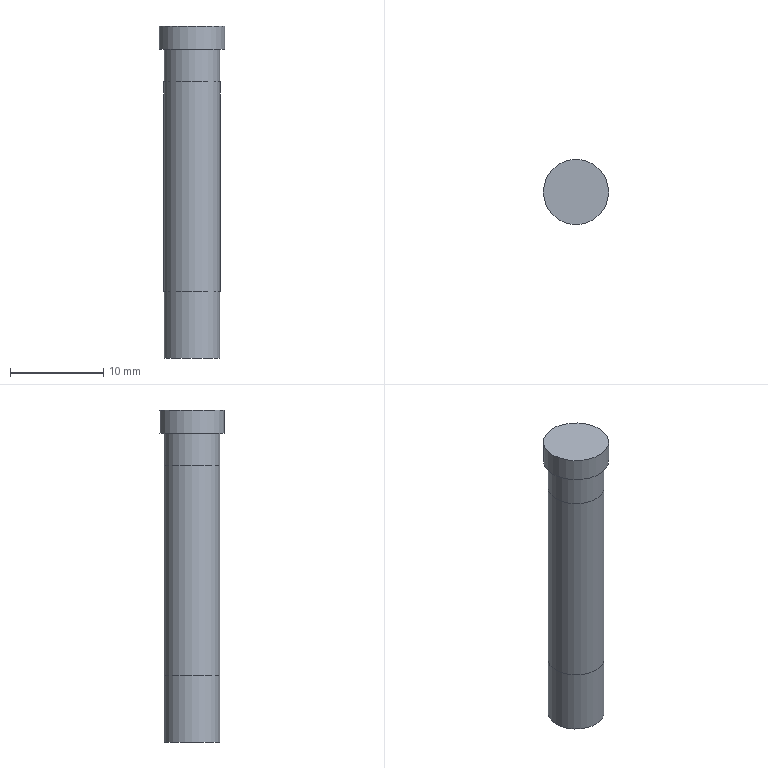Part | NX | features BREP 2 | 2 solids | 10 faces | box 7 x 7 x 35.6 mm | volume 1730 mm3 | plane 5 | cylinder 3 | torus 1 | cone 1 | commonest cylinder face diameters 6 x1 6.008 x1 7 x1
STEP:
#1=CARTESIAN_POINT('',(3.5,0.,-2.5));
#2=VERTEX_POINT('',#1);
#3=CARTESIAN_POINT('',(0.,0.,-2.5));
#4=DIRECTION('',(0.,0.,1.));
#5=DIRECTION('',(1.,0.,0.));
#6=AXIS2_PLACEMENT_3D('',#3,#4,#5);
#7=CIRCLE('',#6,3.5);
#8=EDGE_CURVE('',#2,#2,#7,.T.);
#9=ORIENTED_EDGE('',*,*,#8,.T.);
#10=EDGE_LOOP('',(#9));
#11=FACE_BOUND('',#10,.T.);
#12=CARTESIAN_POINT('',(3.5,0.,0.));
#13=VERTEX_POINT('',#12);
#14=CARTESIAN_POINT('',(0.,0.,0.));
#15=DIRECTION('',(0.,0.,1.));
#16=DIRECTION('',(1.,0.,0.));
#17=AXIS2_PLACEMENT_3D('',#14,#15,#16);
#18=CIRCLE('',#17,3.5);
#19=EDGE_CURVE('',#13,#13,#18,.T.);
#20=ORIENTED_EDGE('',*,*,#19,.F.);
#21=EDGE_LOOP('',(#20));
#22=FACE_BOUND('',#21,.T.);
#23=CARTESIAN_POINT('',(0.,0.,-2.5));
#24=DIRECTION('',(0.,0.,1.));
#25=DIRECTION('',(-1.,0.,0.));
#26=AXIS2_PLACEMENT_3D('',#23,#24,#25);
#27=CYLINDRICAL_SURFACE('',#26,3.5);
#28=ADVANCED_FACE('',(#11,#22),#27,.T.);
#29=CARTESIAN_POINT('',(-3.,0.,-2.5));
#30=VERTEX_POINT('',#29);
#31=CARTESIAN_POINT('',(0.,0.,-2.5));
#32=DIRECTION('',(0.,0.,-1.));
#33=DIRECTION('',(-1.,0.,0.));
#34=AXIS2_PLACEMENT_3D('',#31,#32,#33);
#35=CIRCLE('',#34,3.);
#36=EDGE_CURVE('',#30,#30,#35,.T.);
#37=ORIENTED_EDGE('',*,*,#36,.F.);
#38=EDGE_LOOP('',(#37));
#39=FACE_BOUND('',#38,.T.);
#40=ORIENTED_EDGE('',*,*,#8,.F.);
#41=EDGE_LOOP('',(#40));
#42=FACE_BOUND('',#41,.T.);
#43=CARTESIAN_POINT('',(0.,0.,-2.5));
#44=DIRECTION('',(0.,0.,1.));
#45=DIRECTION('',(-1.,0.,0.));
#46=AXIS2_PLACEMENT_3D('',#43,#44,#45);
#47=PLANE('',#46);
#48=ADVANCED_FACE('',(#39,#42),#47,.F.);
#49=ORIENTED_EDGE('',*,*,#19,.T.);
#50=EDGE_LOOP('',(#49));
#51=FACE_BOUND('',#50,.T.);
#52=CARTESIAN_POINT('',(0.,0.,0.));
#53=DIRECTION('',(0.,0.,1.));
#54=DIRECTION('',(-1.,0.,0.));
#55=AXIS2_PLACEMENT_3D('',#52,#53,#54);
#56=PLANE('',#55);
#57=ADVANCED_FACE('',(#51),#56,.T.);
#58=ORIENTED_EDGE('',*,*,#36,.T.);
#59=EDGE_LOOP('',(#58));
#60=FACE_BOUND('',#59,.T.);
#61=CARTESIAN_POINT('',(-3.,0.,-35.6));
#62=VERTEX_POINT('',#61);
#63=CARTESIAN_POINT('',(0.,0.,-35.6));
#64=DIRECTION('',(0.,0.,-1.));
#65=DIRECTION('',(-1.,0.,0.));
#66=AXIS2_PLACEMENT_3D('',#63,#64,#65);
#67=CIRCLE('',#66,3.);
#68=EDGE_CURVE('',#62,#62,#67,.T.);
#69=ORIENTED_EDGE('',*,*,#68,.F.);
#70=EDGE_LOOP('',(#69));
#71=FACE_BOUND('',#70,.T.);
#72=CARTESIAN_POINT('',(0.,0.,-2.5));
#73=DIRECTION('',(0.,0.,-1.));
#74=DIRECTION('',(1.,0.,0.));
#75=AXIS2_PLACEMENT_3D('',#72,#73,#74);
#76=CYLINDRICAL_SURFACE('',#75,3.);
#77=ADVANCED_FACE('',(#60,#71),#76,.T.);
#78=ORIENTED_EDGE('',*,*,#68,.T.);
#79=EDGE_LOOP('',(#78));
#80=FACE_BOUND('',#79,.T.);
#81=CARTESIAN_POINT('',(0.,0.,-35.6));
#82=DIRECTION('',(0.,0.,-1.));
#83=DIRECTION('',(1.,0.,0.));
#84=AXIS2_PLACEMENT_3D('',#81,#82,#83);
#85=PLANE('',#84);
#86=ADVANCED_FACE('',(#80),#85,.T.);
#87=CLOSED_SHELL('',(#28,#48,#57,#77,#86));
#88=MANIFOLD_SOLID_BREP('',#87);
#89=CARTESIAN_POINT('',(3.004,0.,-28.5));
#90=VERTEX_POINT('',#89);
#91=CARTESIAN_POINT('',(0.,0.,-28.5));
#92=DIRECTION('',(0.,0.,1.));
#93=DIRECTION('',(1.,0.,0.));
#94=AXIS2_PLACEMENT_3D('',#91,#92,#93);
#95=CIRCLE('',#94,3.004);
#96=EDGE_CURVE('',#90,#90,#95,.T.);
#97=ORIENTED_EDGE('',*,*,#96,.T.);
#98=EDGE_LOOP('',(#97));
#99=FACE_BOUND('',#98,.T.);
#100=CARTESIAN_POINT('',(3.004,0.,-6.));
#101=VERTEX_POINT('',#100);
#102=CARTESIAN_POINT('',(0.,0.,-6.));
#103=DIRECTION('',(0.,0.,-1.));
#104=DIRECTION('',(1.,0.,0.));
#105=AXIS2_PLACEMENT_3D('',#102,#103,#104);
#106=CIRCLE('',#105,3.004);
#107=EDGE_CURVE('',#101,#101,#106,.T.);
#108=ORIENTED_EDGE('',*,*,#107,.T.);
#109=EDGE_LOOP('',(#108));
#110=FACE_BOUND('',#109,.T.);
#111=CARTESIAN_POINT('',(0.,0.,-29.5));
#112=DIRECTION('',(0.,0.,1.));
#113=DIRECTION('',(-1.,0.,0.));
#114=AXIS2_PLACEMENT_3D('',#111,#112,#113);
#115=CYLINDRICAL_SURFACE('',#114,3.004);
#116=ADVANCED_FACE('',(#99,#110),#115,.T.);
#117=CARTESIAN_POINT('',(2.736,0.,-29.5));
#118=VERTEX_POINT('',#117);
#119=CARTESIAN_POINT('',(0.,0.,-29.5));
#120=DIRECTION('',(0.,0.,-1.));
#121=DIRECTION('',(1.,0.,0.));
#122=AXIS2_PLACEMENT_3D('',#119,#120,#121);
#123=CIRCLE('',#122,2.736);
#124=EDGE_CURVE('',#118,#118,#123,.T.);
#125=ORIENTED_EDGE('',*,*,#124,.T.);
#126=EDGE_LOOP('',(#125));
#127=FACE_BOUND('',#126,.T.);
#128=CARTESIAN_POINT('',(0.,0.,-29.5));
#129=DIRECTION('',(0.,0.,1.));
#130=DIRECTION('',(-1.,0.,0.));
#131=AXIS2_PLACEMENT_3D('',#128,#129,#130);
#132=PLANE('',#131);
#133=ADVANCED_FACE('',(#127),#132,.F.);
#134=CARTESIAN_POINT('',(1.504,0.,-4.5));
#135=VERTEX_POINT('',#134);
#136=CARTESIAN_POINT('',(0.,0.,-4.5));
#137=DIRECTION('',(0.,0.,1.));
#138=DIRECTION('',(1.,0.,0.));
#139=AXIS2_PLACEMENT_3D('',#136,#137,#138);
#140=CIRCLE('',#139,1.504);
#141=EDGE_CURVE('',#135,#135,#140,.T.);
#142=ORIENTED_EDGE('',*,*,#141,.T.);
#143=EDGE_LOOP('',(#142));
#144=FACE_BOUND('',#143,.T.);
#145=CARTESIAN_POINT('',(0.,0.,-4.5));
#146=DIRECTION('',(0.,0.,1.));
#147=DIRECTION('',(-1.,0.,0.));
#148=AXIS2_PLACEMENT_3D('',#145,#146,#147);
#149=PLANE('',#148);
#150=ADVANCED_FACE('',(#144),#149,.T.);
#151=ORIENTED_EDGE('',*,*,#107,.F.);
#152=EDGE_LOOP('',(#151));
#153=FACE_BOUND('',#152,.T.);
#154=ORIENTED_EDGE('',*,*,#141,.F.);
#155=EDGE_LOOP('',(#154));
#156=FACE_BOUND('',#155,.T.);
#157=CARTESIAN_POINT('',(0.,0.,-6.));
#158=DIRECTION('',(0.,0.,1.));
#159=DIRECTION('',(-1.,0.,0.));
#160=AXIS2_PLACEMENT_3D('',#157,#158,#159);
#161=TOROIDAL_SURFACE('',#160,1.504,1.5);
#162=ADVANCED_FACE('',(#153,#156),#161,.T.);
#163=ORIENTED_EDGE('',*,*,#124,.F.);
#164=EDGE_LOOP('',(#163));
#165=FACE_BOUND('',#164,.T.);
#166=ORIENTED_EDGE('',*,*,#96,.F.);
#167=EDGE_LOOP('',(#166));
#168=FACE_BOUND('',#167,.T.);
#169=CARTESIAN_POINT('',(0.,0.,-28.5));
#170=DIRECTION('',(0.,0.,1.));
#171=DIRECTION('',(-1.,0.,0.));
#172=AXIS2_PLACEMENT_3D('',#169,#170,#171);
#173=CONICAL_SURFACE('',#172,3.004,0.2618);
#174=ADVANCED_FACE('',(#165,#168),#173,.T.);
#175=CLOSED_SHELL('',(#116,#133,#150,#162,#174));
#176=MANIFOLD_SOLID_BREP('',#175);
#177=(LENGTH_UNIT()NAMED_UNIT(*)SI_UNIT(.MILLI.,.METRE.));
#178=UNCERTAINTY_MEASURE_WITH_UNIT(LENGTH_MEASURE(0.00001),#177,'','');
#179=(NAMED_UNIT(*)PLANE_ANGLE_UNIT()SI_UNIT($,.RADIAN.));
#180=(NAMED_UNIT(*)SI_UNIT($,.STERADIAN.)SOLID_ANGLE_UNIT());
#181=(GEOMETRIC_REPRESENTATION_CONTEXT(3)GLOBAL_UNCERTAINTY_ASSIGNED_CONTEXT((#178))GLOBAL_UNIT_ASSIGNED_CONTEXT((#177,#179,#180))REPRESENTATION_CONTEXT('',''));
#182=ADVANCED_BREP_SHAPE_REPRESENTATION('',(#88,#176),#181);